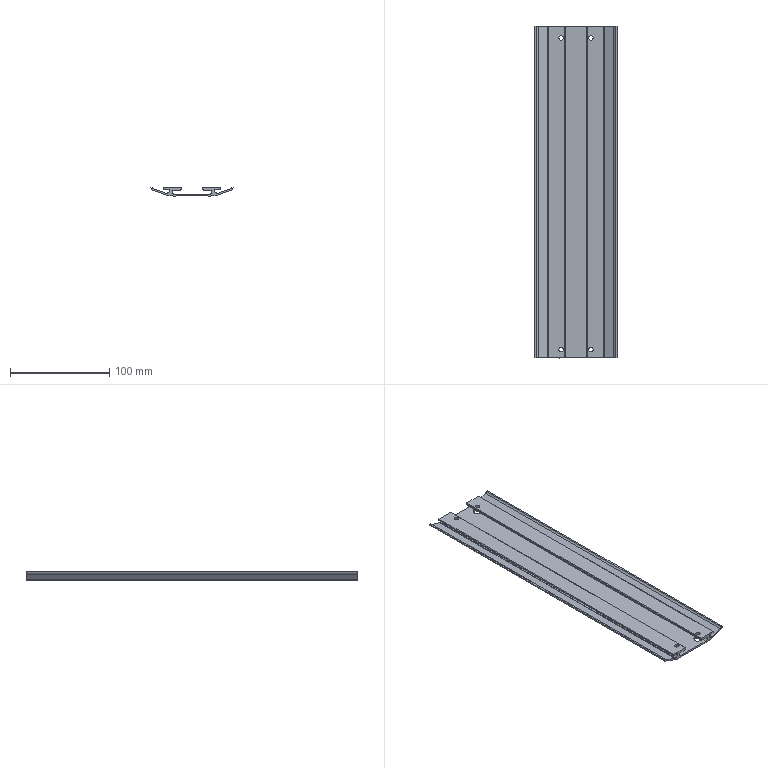Part | SolidWorks | features BaseBody 1 | 1 solid | 79 faces | box 82.5 x 334 x 8.7 mm | volume 80216 mm3 | cylinder 41 | plane 38 | commonest cylinder face diameters 8 x11 1 x8 4.5 x8 6 x6 6.02 x4 1.6 x2